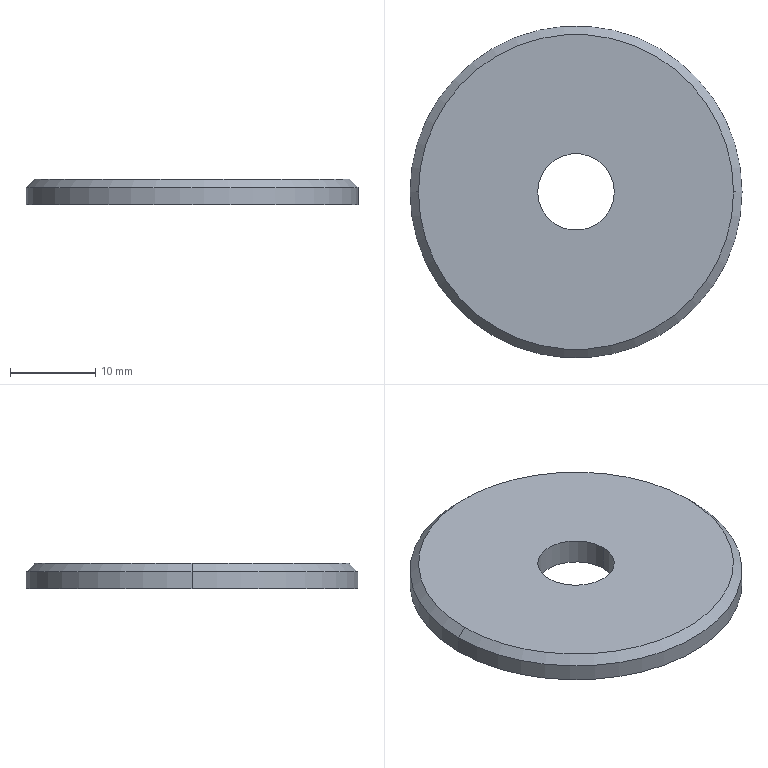Part | STEP file | PODKLADKA_Fi39V11 | 1 solid | 8 faces | box 39 x 39 x 3 mm | volume 3333 mm3 | cylinder 4 | cone 2 | plane 2 | commonest cylinder face diameters 9 x2 39 x2
STEP:
#1=CARTESIAN_POINT('',(0.,0.,0.));
#2=DIRECTION('',(0.,0.,1.));
#3=DIRECTION('',(1.,0.,0.));
#4=AXIS2_PLACEMENT_3D('',#1,#2,#3);
#5=CARTESIAN_POINT('',(18.5,0.,3.));
#6=VERTEX_POINT('',#5);
#7=CARTESIAN_POINT('',(-18.5,0.,3.));
#8=VERTEX_POINT('',#7);
#9=CARTESIAN_POINT('',(0.,0.,3.));
#10=DIRECTION('',(0.,0.,1.));
#11=DIRECTION('',(1.,0.,0.));
#12=AXIS2_PLACEMENT_3D('',#9,#10,#11);
#13=CIRCLE('',#12,18.5);
#14=CARTESIAN_POINT('',(0.,0.,3.));
#15=DIRECTION('',(0.,0.,-1.));
#16=DIRECTION('',(-1.,0.,0.));
#17=AXIS2_PLACEMENT_3D('',#14,#15,#16);
#18=CONICAL_SURFACE('',#17,18.5,0.7854);
#19=CARTESIAN_POINT('',(3.142,0.));
#20=DIRECTION('',(-1.,0.));
#21=VECTOR('',#20,1.);
#22=LINE('',#19,#21);
#23=(GEOMETRIC_REPRESENTATION_CONTEXT(2)PARAMETRIC_REPRESENTATION_CONTEXT()REPRESENTATION_CONTEXT('',''));
#24=DEFINITIONAL_REPRESENTATION('',(#22),#23);
#25=PCURVE('',#18,#24);
#26=CARTESIAN_POINT('',(0.,0.,3.));
#27=DIRECTION('',(0.,0.,1.));
#28=DIRECTION('',(1.,0.,0.));
#29=AXIS2_PLACEMENT_3D('',#26,#27,#28);
#30=PLANE('',#29);
#31=CARTESIAN_POINT('',(0.,0.));
#32=DIRECTION('',(1.,0.));
#33=AXIS2_PLACEMENT_2D('',#31,#32);
#34=CIRCLE('',#33,18.5);
#35=(GEOMETRIC_REPRESENTATION_CONTEXT(2)PARAMETRIC_REPRESENTATION_CONTEXT()REPRESENTATION_CONTEXT('',''));
#36=DEFINITIONAL_REPRESENTATION('',(#34),#35);
#37=PCURVE('',#30,#36);
#38=SURFACE_CURVE('',#13,(#25,#37),.PCURVE_S1.);
#39=EDGE_CURVE('',#6,#8,#38,.T.);
#40=ORIENTED_EDGE('',*,*,#39,.F.);
#41=CARTESIAN_POINT('',(19.5,0.,2.));
#42=VERTEX_POINT('',#41);
#43=CARTESIAN_POINT('',(18.5,0.,3.));
#44=DIRECTION('',(0.7071,0.,-0.7071));
#45=VECTOR('',#44,1.);
#46=LINE('',#43,#45);
#47=CARTESIAN_POINT('',(3.142,0.));
#48=DIRECTION('',(0.,1.));
#49=VECTOR('',#48,1.);
#50=LINE('',#47,#49);
#51=(GEOMETRIC_REPRESENTATION_CONTEXT(2)PARAMETRIC_REPRESENTATION_CONTEXT()REPRESENTATION_CONTEXT('',''));
#52=DEFINITIONAL_REPRESENTATION('',(#50),#51);
#53=PCURVE('',#18,#52);
#54=CARTESIAN_POINT('',(0.,0.,3.));
#55=DIRECTION('',(0.,0.,-1.));
#56=DIRECTION('',(-1.,0.,0.));
#57=AXIS2_PLACEMENT_3D('',#54,#55,#56);
#58=CONICAL_SURFACE('',#57,18.5,0.7854);
#59=CARTESIAN_POINT('',(3.142,0.));
#60=DIRECTION('',(0.,1.));
#61=VECTOR('',#60,1.);
#62=LINE('',#59,#61);
#63=(GEOMETRIC_REPRESENTATION_CONTEXT(2)PARAMETRIC_REPRESENTATION_CONTEXT()REPRESENTATION_CONTEXT('',''));
#64=DEFINITIONAL_REPRESENTATION('',(#62),#63);
#65=PCURVE('',#58,#64);
#66=SURFACE_CURVE('',#46,(#53,#65),.PCURVE_S1.);
#67=EDGE_CURVE('',#6,#42,#66,.T.);
#68=ORIENTED_EDGE('',*,*,#67,.T.);
#69=CARTESIAN_POINT('',(-19.5,0.,2.));
#70=VERTEX_POINT('',#69);
#71=CARTESIAN_POINT('',(0.,0.,2.));
#72=DIRECTION('',(0.,0.,-1.));
#73=DIRECTION('',(1.,0.,0.));
#74=AXIS2_PLACEMENT_3D('',#71,#72,#73);
#75=CIRCLE('',#74,19.5);
#76=CARTESIAN_POINT('',(-3.142,1.));
#77=DIRECTION('',(1.,0.));
#78=VECTOR('',#77,1.);
#79=LINE('',#76,#78);
#80=(GEOMETRIC_REPRESENTATION_CONTEXT(2)PARAMETRIC_REPRESENTATION_CONTEXT()REPRESENTATION_CONTEXT('',''));
#81=DEFINITIONAL_REPRESENTATION('',(#79),#80);
#82=PCURVE('',#18,#81);
#83=CARTESIAN_POINT('',(0.,0.,3.));
#84=DIRECTION('',(0.,0.,-1.));
#85=DIRECTION('',(-1.,0.,0.));
#86=AXIS2_PLACEMENT_3D('',#83,#84,#85);
#87=CYLINDRICAL_SURFACE('',#86,19.5);
#88=CARTESIAN_POINT('',(-3.142,1.));
#89=DIRECTION('',(1.,0.));
#90=VECTOR('',#89,1.);
#91=LINE('',#88,#90);
#92=(GEOMETRIC_REPRESENTATION_CONTEXT(2)PARAMETRIC_REPRESENTATION_CONTEXT()REPRESENTATION_CONTEXT('',''));
#93=DEFINITIONAL_REPRESENTATION('',(#91),#92);
#94=PCURVE('',#87,#93);
#95=SURFACE_CURVE('',#75,(#82,#94),.PCURVE_S1.);
#96=EDGE_CURVE('',#70,#42,#95,.T.);
#97=ORIENTED_EDGE('',*,*,#96,.F.);
#98=CARTESIAN_POINT('',(-18.5,0.,3.));
#99=DIRECTION('',(-0.7071,0.,-0.7071));
#100=VECTOR('',#99,1.);
#101=LINE('',#98,#100);
#102=CARTESIAN_POINT('',(0.,0.));
#103=DIRECTION('',(0.,1.));
#104=VECTOR('',#103,1.);
#105=LINE('',#102,#104);
#106=(GEOMETRIC_REPRESENTATION_CONTEXT(2)PARAMETRIC_REPRESENTATION_CONTEXT()REPRESENTATION_CONTEXT('',''));
#107=DEFINITIONAL_REPRESENTATION('',(#105),#106);
#108=PCURVE('',#18,#107);
#109=CARTESIAN_POINT('',(6.283,0.));
#110=DIRECTION('',(0.,1.));
#111=VECTOR('',#110,1.);
#112=LINE('',#109,#111);
#113=(GEOMETRIC_REPRESENTATION_CONTEXT(2)PARAMETRIC_REPRESENTATION_CONTEXT()REPRESENTATION_CONTEXT('',''));
#114=DEFINITIONAL_REPRESENTATION('',(#112),#113);
#115=PCURVE('',#58,#114);
#116=SURFACE_CURVE('',#101,(#108,#115),.PCURVE_S1.);
#117=EDGE_CURVE('',#8,#70,#116,.T.);
#118=ORIENTED_EDGE('',*,*,#117,.F.);
#119=EDGE_LOOP('',(#40,#68,#97,#118));
#120=FACE_BOUND('',#119,.T.);
#121=ADVANCED_FACE('',(#120),#18,.T.);
#122=CARTESIAN_POINT('',(-4.5,0.,3.));
#123=VERTEX_POINT('',#122);
#124=CARTESIAN_POINT('',(-4.5,0.,0.));
#125=VERTEX_POINT('',#124);
#126=CARTESIAN_POINT('',(-4.5,0.,3.));
#127=DIRECTION('',(0.,0.,-1.));
#128=VECTOR('',#127,1.);
#129=LINE('',#126,#128);
#130=CARTESIAN_POINT('',(0.,0.,3.));
#131=DIRECTION('',(0.,0.,-1.));
#132=DIRECTION('',(-1.,0.,0.));
#133=AXIS2_PLACEMENT_3D('',#130,#131,#132);
#134=CYLINDRICAL_SURFACE('',#133,4.5);
#135=CARTESIAN_POINT('',(6.283,0.));
#136=DIRECTION('',(0.,1.));
#137=VECTOR('',#136,1.);
#138=LINE('',#135,#137);
#139=(GEOMETRIC_REPRESENTATION_CONTEXT(2)PARAMETRIC_REPRESENTATION_CONTEXT()REPRESENTATION_CONTEXT('',''));
#140=DEFINITIONAL_REPRESENTATION('',(#138),#139);
#141=PCURVE('',#134,#140);
#142=CARTESIAN_POINT('',(0.,0.,3.));
#143=DIRECTION('',(0.,0.,-1.));
#144=DIRECTION('',(-1.,0.,0.));
#145=AXIS2_PLACEMENT_3D('',#142,#143,#144);
#146=CYLINDRICAL_SURFACE('',#145,4.5);
#147=CARTESIAN_POINT('',(0.,0.));
#148=DIRECTION('',(0.,1.));
#149=VECTOR('',#148,1.);
#150=LINE('',#147,#149);
#151=(GEOMETRIC_REPRESENTATION_CONTEXT(2)PARAMETRIC_REPRESENTATION_CONTEXT()REPRESENTATION_CONTEXT('',''));
#152=DEFINITIONAL_REPRESENTATION('',(#150),#151);
#153=PCURVE('',#146,#152);
#154=SURFACE_CURVE('',#129,(#141,#153),.PCURVE_S1.);
#155=EDGE_CURVE('',#123,#125,#154,.T.);
#156=ORIENTED_EDGE('',*,*,#155,.T.);
#157=CARTESIAN_POINT('',(4.5,0.,0.));
#158=VERTEX_POINT('',#157);
#159=CARTESIAN_POINT('',(0.,0.,0.));
#160=DIRECTION('',(0.,0.,1.));
#161=DIRECTION('',(1.,0.,0.));
#162=AXIS2_PLACEMENT_3D('',#159,#160,#161);
#163=CIRCLE('',#162,4.5);
#164=CARTESIAN_POINT('',(9.425,3.));
#165=DIRECTION('',(-1.,0.));
#166=VECTOR('',#165,1.);
#167=LINE('',#164,#166);
#168=(GEOMETRIC_REPRESENTATION_CONTEXT(2)PARAMETRIC_REPRESENTATION_CONTEXT()REPRESENTATION_CONTEXT('',''));
#169=DEFINITIONAL_REPRESENTATION('',(#167),#168);
#170=PCURVE('',#134,#169);
#171=CARTESIAN_POINT('',(0.,0.,0.));
#172=DIRECTION('',(0.,0.,1.));
#173=DIRECTION('',(1.,0.,0.));
#174=AXIS2_PLACEMENT_3D('',#171,#172,#173);
#175=PLANE('',#174);
#176=CARTESIAN_POINT('',(0.,0.));
#177=DIRECTION('',(1.,0.));
#178=AXIS2_PLACEMENT_2D('',#176,#177);
#179=CIRCLE('',#178,4.5);
#180=(GEOMETRIC_REPRESENTATION_CONTEXT(2)PARAMETRIC_REPRESENTATION_CONTEXT()REPRESENTATION_CONTEXT('',''));
#181=DEFINITIONAL_REPRESENTATION('',(#179),#180);
#182=PCURVE('',#175,#181);
#183=SURFACE_CURVE('',#163,(#170,#182),.PCURVE_S1.);
#184=EDGE_CURVE('',#125,#158,#183,.T.);
#185=ORIENTED_EDGE('',*,*,#184,.T.);
#186=CARTESIAN_POINT('',(4.5,0.,3.));
#187=VERTEX_POINT('',#186);
#188=CARTESIAN_POINT('',(4.5,0.,3.));
#189=DIRECTION('',(0.,0.,-1.));
#190=VECTOR('',#189,1.);
#191=LINE('',#188,#190);
#192=CARTESIAN_POINT('',(3.142,0.));
#193=DIRECTION('',(0.,1.));
#194=VECTOR('',#193,1.);
#195=LINE('',#192,#194);
#196=(GEOMETRIC_REPRESENTATION_CONTEXT(2)PARAMETRIC_REPRESENTATION_CONTEXT()REPRESENTATION_CONTEXT('',''));
#197=DEFINITIONAL_REPRESENTATION('',(#195),#196);
#198=PCURVE('',#134,#197);
#199=CARTESIAN_POINT('',(3.142,0.));
#200=DIRECTION('',(0.,1.));
#201=VECTOR('',#200,1.);
#202=LINE('',#199,#201);
#203=(GEOMETRIC_REPRESENTATION_CONTEXT(2)PARAMETRIC_REPRESENTATION_CONTEXT()REPRESENTATION_CONTEXT('',''));
#204=DEFINITIONAL_REPRESENTATION('',(#202),#203);
#205=PCURVE('',#146,#204);
#206=SURFACE_CURVE('',#191,(#198,#205),.PCURVE_S1.);
#207=EDGE_CURVE('',#187,#158,#206,.T.);
#208=ORIENTED_EDGE('',*,*,#207,.F.);
#209=CARTESIAN_POINT('',(0.,0.,3.));
#210=DIRECTION('',(0.,0.,1.));
#211=DIRECTION('',(1.,0.,0.));
#212=AXIS2_PLACEMENT_3D('',#209,#210,#211);
#213=CIRCLE('',#212,4.5);
#214=CARTESIAN_POINT('',(9.425,0.));
#215=DIRECTION('',(-1.,0.));
#216=VECTOR('',#215,1.);
#217=LINE('',#214,#216);
#218=(GEOMETRIC_REPRESENTATION_CONTEXT(2)PARAMETRIC_REPRESENTATION_CONTEXT()REPRESENTATION_CONTEXT('',''));
#219=DEFINITIONAL_REPRESENTATION('',(#217),#218);
#220=PCURVE('',#134,#219);
#221=CARTESIAN_POINT('',(0.,0.));
#222=DIRECTION('',(1.,0.));
#223=AXIS2_PLACEMENT_2D('',#221,#222);
#224=CIRCLE('',#223,4.5);
#225=(GEOMETRIC_REPRESENTATION_CONTEXT(2)PARAMETRIC_REPRESENTATION_CONTEXT()REPRESENTATION_CONTEXT('',''));
#226=DEFINITIONAL_REPRESENTATION('',(#224),#225);
#227=PCURVE('',#30,#226);
#228=SURFACE_CURVE('',#213,(#220,#227),.PCURVE_S1.);
#229=EDGE_CURVE('',#123,#187,#228,.T.);
#230=ORIENTED_EDGE('',*,*,#229,.F.);
#231=EDGE_LOOP('',(#156,#185,#208,#230));
#232=FACE_BOUND('',#231,.F.);
#233=ADVANCED_FACE('',(#232),#134,.F.);
#234=ORIENTED_EDGE('',*,*,#96,.T.);
#235=CARTESIAN_POINT('',(19.5,0.,0.));
#236=VERTEX_POINT('',#235);
#237=CARTESIAN_POINT('',(19.5,0.,3.));
#238=DIRECTION('',(0.,0.,-1.));
#239=VECTOR('',#238,1.);
#240=LINE('',#237,#239);
#241=CARTESIAN_POINT('',(3.142,0.));
#242=DIRECTION('',(0.,1.));
#243=VECTOR('',#242,1.);
#244=LINE('',#241,#243);
#245=(GEOMETRIC_REPRESENTATION_CONTEXT(2)PARAMETRIC_REPRESENTATION_CONTEXT()REPRESENTATION_CONTEXT('',''));
#246=DEFINITIONAL_REPRESENTATION('',(#244),#245);
#247=PCURVE('',#87,#246);
#248=CARTESIAN_POINT('',(0.,0.,3.));
#249=DIRECTION('',(0.,0.,-1.));
#250=DIRECTION('',(-1.,0.,0.));
#251=AXIS2_PLACEMENT_3D('',#248,#249,#250);
#252=CYLINDRICAL_SURFACE('',#251,19.5);
#253=CARTESIAN_POINT('',(3.142,0.));
#254=DIRECTION('',(0.,1.));
#255=VECTOR('',#254,1.);
#256=LINE('',#253,#255);
#257=(GEOMETRIC_REPRESENTATION_CONTEXT(2)PARAMETRIC_REPRESENTATION_CONTEXT()REPRESENTATION_CONTEXT('',''));
#258=DEFINITIONAL_REPRESENTATION('',(#256),#257);
#259=PCURVE('',#252,#258);
#260=SURFACE_CURVE('',#240,(#247,#259),.PCURVE_S1.);
#261=EDGE_CURVE('',#42,#236,#260,.T.);
#262=ORIENTED_EDGE('',*,*,#261,.T.);
#263=CARTESIAN_POINT('',(-19.5,0.,0.));
#264=VERTEX_POINT('',#263);
#265=CARTESIAN_POINT('',(0.,0.,0.));
#266=DIRECTION('',(0.,0.,1.));
#267=DIRECTION('',(1.,0.,0.));
#268=AXIS2_PLACEMENT_3D('',#265,#266,#267);
#269=CIRCLE('',#268,19.5);
#270=CARTESIAN_POINT('',(3.142,3.));
#271=DIRECTION('',(-1.,0.));
#272=VECTOR('',#271,1.);
#273=LINE('',#270,#272);
#274=(GEOMETRIC_REPRESENTATION_CONTEXT(2)PARAMETRIC_REPRESENTATION_CONTEXT()REPRESENTATION_CONTEXT('',''));
#275=DEFINITIONAL_REPRESENTATION('',(#273),#274);
#276=PCURVE('',#87,#275);
#277=CARTESIAN_POINT('',(0.,0.));
#278=DIRECTION('',(1.,0.));
#279=AXIS2_PLACEMENT_2D('',#277,#278);
#280=CIRCLE('',#279,19.5);
#281=(GEOMETRIC_REPRESENTATION_CONTEXT(2)PARAMETRIC_REPRESENTATION_CONTEXT()REPRESENTATION_CONTEXT('',''));
#282=DEFINITIONAL_REPRESENTATION('',(#280),#281);
#283=PCURVE('',#175,#282);
#284=SURFACE_CURVE('',#269,(#276,#283),.PCURVE_S1.);
#285=EDGE_CURVE('',#236,#264,#284,.T.);
#286=ORIENTED_EDGE('',*,*,#285,.T.);
#287=CARTESIAN_POINT('',(-19.5,0.,3.));
#288=DIRECTION('',(0.,0.,-1.));
#289=VECTOR('',#288,1.);
#290=LINE('',#287,#289);
#291=CARTESIAN_POINT('',(0.,0.));
#292=DIRECTION('',(0.,1.));
#293=VECTOR('',#292,1.);
#294=LINE('',#291,#293);
#295=(GEOMETRIC_REPRESENTATION_CONTEXT(2)PARAMETRIC_REPRESENTATION_CONTEXT()REPRESENTATION_CONTEXT('',''));
#296=DEFINITIONAL_REPRESENTATION('',(#294),#295);
#297=PCURVE('',#87,#296);
#298=CARTESIAN_POINT('',(6.283,0.));
#299=DIRECTION('',(0.,1.));
#300=VECTOR('',#299,1.);
#301=LINE('',#298,#300);
#302=(GEOMETRIC_REPRESENTATION_CONTEXT(2)PARAMETRIC_REPRESENTATION_CONTEXT()REPRESENTATION_CONTEXT('',''));
#303=DEFINITIONAL_REPRESENTATION('',(#301),#302);
#304=PCURVE('',#252,#303);
#305=SURFACE_CURVE('',#290,(#297,#304),.PCURVE_S1.);
#306=EDGE_CURVE('',#70,#264,#305,.T.);
#307=ORIENTED_EDGE('',*,*,#306,.F.);
#308=EDGE_LOOP('',(#234,#262,#286,#307));
#309=FACE_BOUND('',#308,.T.);
#310=ADVANCED_FACE('',(#309),#87,.T.);
#311=CARTESIAN_POINT('',(0.,0.,3.));
#312=DIRECTION('',(0.,0.,1.));
#313=DIRECTION('',(1.,0.,0.));
#314=AXIS2_PLACEMENT_3D('',#311,#312,#313);
#315=CIRCLE('',#314,18.5);
#316=CARTESIAN_POINT('',(0.,0.));
#317=DIRECTION('',(1.,0.));
#318=AXIS2_PLACEMENT_2D('',#316,#317);
#319=CIRCLE('',#318,18.5);
#320=(GEOMETRIC_REPRESENTATION_CONTEXT(2)PARAMETRIC_REPRESENTATION_CONTEXT()REPRESENTATION_CONTEXT('',''));
#321=DEFINITIONAL_REPRESENTATION('',(#319),#320);
#322=PCURVE('',#30,#321);
#323=CARTESIAN_POINT('',(9.425,0.));
#324=DIRECTION('',(-1.,0.));
#325=VECTOR('',#324,1.);
#326=LINE('',#323,#325);
#327=(GEOMETRIC_REPRESENTATION_CONTEXT(2)PARAMETRIC_REPRESENTATION_CONTEXT()REPRESENTATION_CONTEXT('',''));
#328=DEFINITIONAL_REPRESENTATION('',(#326),#327);
#329=PCURVE('',#58,#328);
#330=SURFACE_CURVE('',#315,(#322,#329),.PCURVE_S1.);
#331=EDGE_CURVE('',#8,#6,#330,.T.);
#332=ORIENTED_EDGE('',*,*,#331,.T.);
#333=ORIENTED_EDGE('',*,*,#39,.T.);
#334=EDGE_LOOP('',(#332,#333));
#335=FACE_BOUND('',#334,.T.);
#336=ORIENTED_EDGE('',*,*,#229,.F.);
#337=CARTESIAN_POINT('',(0.,0.,3.));
#338=DIRECTION('',(0.,0.,1.));
#339=DIRECTION('',(1.,0.,0.));
#340=AXIS2_PLACEMENT_3D('',#337,#338,#339);
#341=CIRCLE('',#340,4.5);
#342=CARTESIAN_POINT('',(0.,0.));
#343=DIRECTION('',(1.,0.));
#344=AXIS2_PLACEMENT_2D('',#342,#343);
#345=CIRCLE('',#344,4.5);
#346=(GEOMETRIC_REPRESENTATION_CONTEXT(2)PARAMETRIC_REPRESENTATION_CONTEXT()REPRESENTATION_CONTEXT('',''));
#347=DEFINITIONAL_REPRESENTATION('',(#345),#346);
#348=PCURVE('',#30,#347);
#349=CARTESIAN_POINT('',(3.142,0.));
#350=DIRECTION('',(-1.,0.));
#351=VECTOR('',#350,1.);
#352=LINE('',#349,#351);
#353=(GEOMETRIC_REPRESENTATION_CONTEXT(2)PARAMETRIC_REPRESENTATION_CONTEXT()REPRESENTATION_CONTEXT('',''));
#354=DEFINITIONAL_REPRESENTATION('',(#352),#353);
#355=PCURVE('',#146,#354);
#356=SURFACE_CURVE('',#341,(#348,#355),.PCURVE_S1.);
#357=EDGE_CURVE('',#187,#123,#356,.T.);
#358=ORIENTED_EDGE('',*,*,#357,.F.);
#359=EDGE_LOOP('',(#336,#358));
#360=FACE_BOUND('',#359,.T.);
#361=ADVANCED_FACE('',(#335,#360),#30,.T.);
#362=CARTESIAN_POINT('',(0.,0.,0.));
#363=DIRECTION('',(0.,0.,1.));
#364=DIRECTION('',(1.,0.,0.));
#365=AXIS2_PLACEMENT_3D('',#362,#363,#364);
#366=CIRCLE('',#365,19.5);
#367=CARTESIAN_POINT('',(0.,0.));
#368=DIRECTION('',(1.,0.));
#369=AXIS2_PLACEMENT_2D('',#367,#368);
#370=CIRCLE('',#369,19.5);
#371=(GEOMETRIC_REPRESENTATION_CONTEXT(2)PARAMETRIC_REPRESENTATION_CONTEXT()REPRESENTATION_CONTEXT('',''));
#372=DEFINITIONAL_REPRESENTATION('',(#370),#371);
#373=PCURVE('',#175,#372);
#374=CARTESIAN_POINT('',(9.425,3.));
#375=DIRECTION('',(-1.,0.));
#376=VECTOR('',#375,1.);
#377=LINE('',#374,#376);
#378=(GEOMETRIC_REPRESENTATION_CONTEXT(2)PARAMETRIC_REPRESENTATION_CONTEXT()REPRESENTATION_CONTEXT('',''));
#379=DEFINITIONAL_REPRESENTATION('',(#377),#378);
#380=PCURVE('',#252,#379);
#381=SURFACE_CURVE('',#366,(#373,#380),.PCURVE_S1.);
#382=EDGE_CURVE('',#264,#236,#381,.T.);
#383=ORIENTED_EDGE('',*,*,#382,.F.);
#384=ORIENTED_EDGE('',*,*,#285,.F.);
#385=EDGE_LOOP('',(#383,#384));
#386=FACE_BOUND('',#385,.T.);
#387=ORIENTED_EDGE('',*,*,#184,.T.);
#388=CARTESIAN_POINT('',(0.,0.,0.));
#389=DIRECTION('',(0.,0.,1.));
#390=DIRECTION('',(1.,0.,0.));
#391=AXIS2_PLACEMENT_3D('',#388,#389,#390);
#392=CIRCLE('',#391,4.5);
#393=CARTESIAN_POINT('',(0.,0.));
#394=DIRECTION('',(1.,0.));
#395=AXIS2_PLACEMENT_2D('',#393,#394);
#396=CIRCLE('',#395,4.5);
#397=(GEOMETRIC_REPRESENTATION_CONTEXT(2)PARAMETRIC_REPRESENTATION_CONTEXT()REPRESENTATION_CONTEXT('',''));
#398=DEFINITIONAL_REPRESENTATION('',(#396),#397);
#399=PCURVE('',#175,#398);
#400=CARTESIAN_POINT('',(3.142,3.));
#401=DIRECTION('',(-1.,0.));
#402=VECTOR('',#401,1.);
#403=LINE('',#400,#402);
#404=(GEOMETRIC_REPRESENTATION_CONTEXT(2)PARAMETRIC_REPRESENTATION_CONTEXT()REPRESENTATION_CONTEXT('',''));
#405=DEFINITIONAL_REPRESENTATION('',(#403),#404);
#406=PCURVE('',#146,#405);
#407=SURFACE_CURVE('',#392,(#399,#406),.PCURVE_S1.);
#408=EDGE_CURVE('',#158,#125,#407,.T.);
#409=ORIENTED_EDGE('',*,*,#408,.T.);
#410=EDGE_LOOP('',(#387,#409));
#411=FACE_BOUND('',#410,.T.);
#412=ADVANCED_FACE('',(#386,#411),#175,.F.);
#413=ORIENTED_EDGE('',*,*,#261,.F.);
#414=CARTESIAN_POINT('',(0.,0.,2.));
#415=DIRECTION('',(0.,0.,-1.));
#416=DIRECTION('',(1.,0.,0.));
#417=AXIS2_PLACEMENT_3D('',#414,#415,#416);
#418=CIRCLE('',#417,19.5);
#419=CARTESIAN_POINT('',(3.142,1.));
#420=DIRECTION('',(1.,0.));
#421=VECTOR('',#420,1.);
#422=LINE('',#419,#421);
#423=(GEOMETRIC_REPRESENTATION_CONTEXT(2)PARAMETRIC_REPRESENTATION_CONTEXT()REPRESENTATION_CONTEXT('',''));
#424=DEFINITIONAL_REPRESENTATION('',(#422),#423);
#425=PCURVE('',#252,#424);
#426=CARTESIAN_POINT('',(3.142,1.));
#427=DIRECTION('',(1.,0.));
#428=VECTOR('',#427,1.);
#429=LINE('',#426,#428);
#430=(GEOMETRIC_REPRESENTATION_CONTEXT(2)PARAMETRIC_REPRESENTATION_CONTEXT()REPRESENTATION_CONTEXT('',''));
#431=DEFINITIONAL_REPRESENTATION('',(#429),#430);
#432=PCURVE('',#58,#431);
#433=SURFACE_CURVE('',#418,(#425,#432),.PCURVE_S1.);
#434=EDGE_CURVE('',#42,#70,#433,.T.);
#435=ORIENTED_EDGE('',*,*,#434,.T.);
#436=ORIENTED_EDGE('',*,*,#306,.T.);
#437=ORIENTED_EDGE('',*,*,#382,.T.);
#438=EDGE_LOOP('',(#413,#435,#436,#437));
#439=FACE_BOUND('',#438,.T.);
#440=ADVANCED_FACE('',(#439),#252,.T.);
#441=ORIENTED_EDGE('',*,*,#408,.T.);
#442=ORIENTED_EDGE('',*,*,#155,.F.);
#443=ORIENTED_EDGE('',*,*,#357,.F.);
#444=ORIENTED_EDGE('',*,*,#207,.T.);
#445=EDGE_LOOP('',(#441,#442,#443,#444));
#446=FACE_BOUND('',#445,.F.);
#447=ADVANCED_FACE('',(#446),#146,.F.);
#448=ORIENTED_EDGE('',*,*,#67,.F.);
#449=ORIENTED_EDGE('',*,*,#331,.F.);
#450=ORIENTED_EDGE('',*,*,#117,.T.);
#451=ORIENTED_EDGE('',*,*,#434,.F.);
#452=EDGE_LOOP('',(#448,#449,#450,#451));
#453=FACE_BOUND('',#452,.T.);
#454=ADVANCED_FACE('',(#453),#58,.T.);
#455=CLOSED_SHELL('',(#121,#233,#310,#361,#412,#440,#447,#454));
#456=MANIFOLD_SOLID_BREP('',#455);
#457=(LENGTH_UNIT()NAMED_UNIT(*)SI_UNIT(.MILLI.,.METRE.));
#458=UNCERTAINTY_MEASURE_WITH_UNIT(LENGTH_MEASURE(0.0000001),#457,'','');
#459=(NAMED_UNIT(*)PLANE_ANGLE_UNIT()SI_UNIT($,.RADIAN.));
#460=(NAMED_UNIT(*)SI_UNIT($,.STERADIAN.)SOLID_ANGLE_UNIT());
#461=(GEOMETRIC_REPRESENTATION_CONTEXT(3)GLOBAL_UNCERTAINTY_ASSIGNED_CONTEXT((#458))GLOBAL_UNIT_ASSIGNED_CONTEXT((#457,#459,#460))REPRESENTATION_CONTEXT('',''));
#462=ADVANCED_BREP_SHAPE_REPRESENTATION('',(#4,#456),#461);